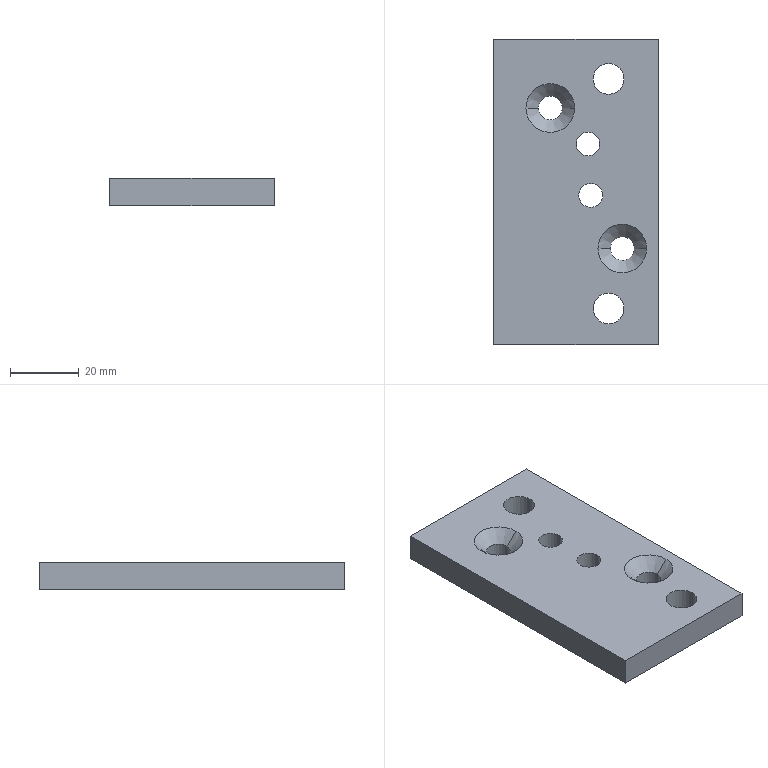Part | 1 solid | 22 faces | box 48 x 89 x 8 mm | volume 31544 mm3 | cylinder 12 | plane 6 | cone 4 | commonest cylinder face diameters 7 x8 9 x4